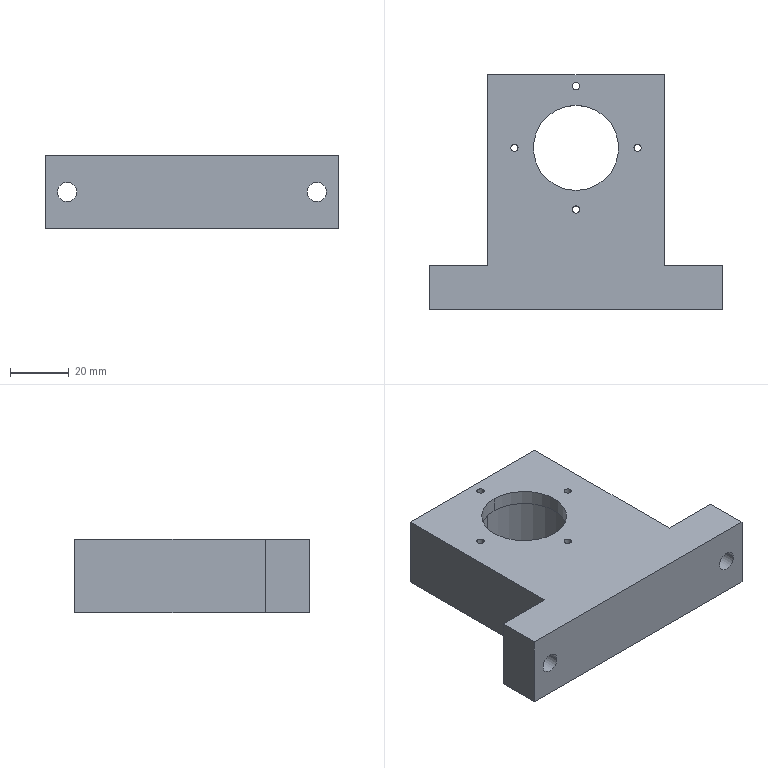Part | SolidWorks | features BaseBody 1 | 1 solid | 37 faces | box 100 x 80 x 25 mm | volume 110111 mm3 | cylinder 20 | plane 13 | cone 4 | commonest cylinder face diameters 2.5 x8 6.6 x4 11 x4 29 x2 35 x2
STEP:
#1=CARTESIAN_POINT('',(-22.25,7.5,25.));
#2=VERTEX_POINT('',#1);
#3=CARTESIAN_POINT('',(-19.75,7.5,25.));
#4=VERTEX_POINT('',#3);
#5=CARTESIAN_POINT('',(-21.,7.5,25.));
#6=DIRECTION('',(0.,0.,1.));
#7=DIRECTION('',(-1.,0.,0.));
#8=AXIS2_PLACEMENT_3D('',#5,#6,#7);
#9=CIRCLE('',#8,1.25);
#10=EDGE_CURVE('',#2,#4,#9,.T.);
#11=ORIENTED_EDGE('',*,*,#10,.T.);
#12=CARTESIAN_POINT('',(-19.75,7.5,0.));
#13=VERTEX_POINT('',#12);
#14=CARTESIAN_POINT('',(-19.75,7.5,25.));
#15=DIRECTION('',(0.,0.,-1.));
#16=VECTOR('',#15,1000.);
#17=LINE('',#14,#16);
#18=EDGE_CURVE('',#4,#13,#17,.T.);
#19=ORIENTED_EDGE('',*,*,#18,.T.);
#20=CARTESIAN_POINT('',(-22.25,7.5,0.));
#21=VERTEX_POINT('',#20);
#22=CARTESIAN_POINT('',(-21.,7.5,0.));
#23=DIRECTION('',(0.,0.,-1.));
#24=DIRECTION('',(-1.,0.,0.));
#25=AXIS2_PLACEMENT_3D('',#22,#23,#24);
#26=CIRCLE('',#25,1.25);
#27=EDGE_CURVE('',#13,#21,#26,.T.);
#28=ORIENTED_EDGE('',*,*,#27,.T.);
#29=CARTESIAN_POINT('',(-22.25,7.5,25.));
#30=DIRECTION('',(0.,0.,-1.));
#31=VECTOR('',#30,1000.);
#32=LINE('',#29,#31);
#33=EDGE_CURVE('',#2,#21,#32,.T.);
#34=ORIENTED_EDGE('',*,*,#33,.F.);
#35=EDGE_LOOP('',(#11,#19,#28,#34));
#36=FACE_OUTER_BOUND('',#35,.T.);
#37=CARTESIAN_POINT('',(-21.,7.5,25.));
#38=DIRECTION('',(0.,0.,-1.));
#39=DIRECTION('',(-1.,0.,0.));
#40=AXIS2_PLACEMENT_3D('',#37,#38,#39);
#41=CYLINDRICAL_SURFACE('',#40,1.25);
#42=ADVANCED_FACE('',(#36),#41,.F.);
#43=CARTESIAN_POINT('',(0.,25.,20.));
#44=VERTEX_POINT('',#43);
#45=CARTESIAN_POINT('',(0.,-10.,20.));
#46=VERTEX_POINT('',#45);
#47=CARTESIAN_POINT('',(0.,7.5,20.));
#48=DIRECTION('',(0.,0.,1.));
#49=DIRECTION('',(0.,1.,0.));
#50=AXIS2_PLACEMENT_3D('',#47,#48,#49);
#51=CIRCLE('',#50,17.5);
#52=EDGE_CURVE('',#44,#46,#51,.T.);
#53=ORIENTED_EDGE('',*,*,#52,.T.);
#54=CARTESIAN_POINT('',(0.,-10.,0.));
#55=VERTEX_POINT('',#54);
#56=CARTESIAN_POINT('',(0.,-10.,20.));
#57=DIRECTION('',(0.,0.,-1.));
#58=VECTOR('',#57,1000.);
#59=LINE('',#56,#58);
#60=EDGE_CURVE('',#46,#55,#59,.T.);
#61=ORIENTED_EDGE('',*,*,#60,.T.);
#62=CARTESIAN_POINT('',(0.,25.,0.));
#63=VERTEX_POINT('',#62);
#64=CARTESIAN_POINT('',(0.,7.5,0.));
#65=DIRECTION('',(0.,0.,-1.));
#66=DIRECTION('',(0.,1.,0.));
#67=AXIS2_PLACEMENT_3D('',#64,#65,#66);
#68=CIRCLE('',#67,17.5);
#69=EDGE_CURVE('',#55,#63,#68,.T.);
#70=ORIENTED_EDGE('',*,*,#69,.T.);
#71=CARTESIAN_POINT('',(0.,25.,20.));
#72=DIRECTION('',(0.,0.,-1.));
#73=VECTOR('',#72,1000.);
#74=LINE('',#71,#73);
#75=EDGE_CURVE('',#44,#63,#74,.T.);
#76=ORIENTED_EDGE('',*,*,#75,.F.);
#77=EDGE_LOOP('',(#53,#61,#70,#76));
#78=FACE_OUTER_BOUND('',#77,.T.);
#79=CARTESIAN_POINT('',(0.,7.5,20.));
#80=DIRECTION('',(0.,0.,-1.));
#81=DIRECTION('',(0.,1.,0.));
#82=AXIS2_PLACEMENT_3D('',#79,#80,#81);
#83=CYLINDRICAL_SURFACE('',#82,17.5);
#84=ADVANCED_FACE('',(#78),#83,.F.);
#85=CARTESIAN_POINT('',(1.25,28.5,25.));
#86=VERTEX_POINT('',#85);
#87=CARTESIAN_POINT('',(-1.25,28.5,25.));
#88=VERTEX_POINT('',#87);
#89=CARTESIAN_POINT('',(0.,28.5,25.));
#90=DIRECTION('',(0.,0.,-1.));
#91=DIRECTION('',(-1.,0.,0.));
#92=AXIS2_PLACEMENT_3D('',#89,#90,#91);
#93=CIRCLE('',#92,1.25);
#94=EDGE_CURVE('',#86,#88,#93,.T.);
#95=ORIENTED_EDGE('',*,*,#94,.F.);
#96=CARTESIAN_POINT('',(1.25,28.5,0.));
#97=VERTEX_POINT('',#96);
#98=CARTESIAN_POINT('',(1.25,28.5,25.));
#99=DIRECTION('',(0.,0.,-1.));
#100=VECTOR('',#99,1000.);
#101=LINE('',#98,#100);
#102=EDGE_CURVE('',#86,#97,#101,.T.);
#103=ORIENTED_EDGE('',*,*,#102,.T.);
#104=CARTESIAN_POINT('',(-1.25,28.5,0.));
#105=VERTEX_POINT('',#104);
#106=CARTESIAN_POINT('',(0.,28.5,0.));
#107=DIRECTION('',(0.,0.,-1.));
#108=DIRECTION('',(-1.,0.,0.));
#109=AXIS2_PLACEMENT_3D('',#106,#107,#108);
#110=CIRCLE('',#109,1.25);
#111=EDGE_CURVE('',#97,#105,#110,.T.);
#112=ORIENTED_EDGE('',*,*,#111,.T.);
#113=CARTESIAN_POINT('',(-1.25,28.5,25.));
#114=DIRECTION('',(0.,0.,-1.));
#115=VECTOR('',#114,1000.);
#116=LINE('',#113,#115);
#117=EDGE_CURVE('',#88,#105,#116,.T.);
#118=ORIENTED_EDGE('',*,*,#117,.F.);
#119=EDGE_LOOP('',(#95,#103,#112,#118));
#120=FACE_OUTER_BOUND('',#119,.T.);
#121=CARTESIAN_POINT('',(0.,28.5,25.));
#122=DIRECTION('',(0.,0.,-1.));
#123=DIRECTION('',(-1.,0.,0.));
#124=AXIS2_PLACEMENT_3D('',#121,#122,#123);
#125=CYLINDRICAL_SURFACE('',#124,1.25);
#126=ADVANCED_FACE('',(#120),#125,.F.);
#127=CARTESIAN_POINT('',(22.25,7.5,25.));
#128=VERTEX_POINT('',#127);
#129=CARTESIAN_POINT('',(19.75,7.5,25.));
#130=VERTEX_POINT('',#129);
#131=CARTESIAN_POINT('',(21.,7.5,25.));
#132=DIRECTION('',(0.,0.,-1.));
#133=DIRECTION('',(-1.,0.,0.));
#134=AXIS2_PLACEMENT_3D('',#131,#132,#133);
#135=CIRCLE('',#134,1.25);
#136=EDGE_CURVE('',#128,#130,#135,.T.);
#137=ORIENTED_EDGE('',*,*,#136,.F.);
#138=CARTESIAN_POINT('',(22.25,7.5,0.));
#139=VERTEX_POINT('',#138);
#140=CARTESIAN_POINT('',(22.25,7.5,25.));
#141=DIRECTION('',(0.,0.,-1.));
#142=VECTOR('',#141,1000.);
#143=LINE('',#140,#142);
#144=EDGE_CURVE('',#128,#139,#143,.T.);
#145=ORIENTED_EDGE('',*,*,#144,.T.);
#146=CARTESIAN_POINT('',(19.75,7.5,0.));
#147=VERTEX_POINT('',#146);
#148=CARTESIAN_POINT('',(21.,7.5,0.));
#149=DIRECTION('',(0.,0.,-1.));
#150=DIRECTION('',(-1.,0.,0.));
#151=AXIS2_PLACEMENT_3D('',#148,#149,#150);
#152=CIRCLE('',#151,1.25);
#153=EDGE_CURVE('',#139,#147,#152,.T.);
#154=ORIENTED_EDGE('',*,*,#153,.T.);
#155=CARTESIAN_POINT('',(19.75,7.5,25.));
#156=DIRECTION('',(0.,0.,-1.));
#157=VECTOR('',#156,1000.);
#158=LINE('',#155,#157);
#159=EDGE_CURVE('',#130,#147,#158,.T.);
#160=ORIENTED_EDGE('',*,*,#159,.F.);
#161=EDGE_LOOP('',(#137,#145,#154,#160));
#162=FACE_OUTER_BOUND('',#161,.T.);
#163=CARTESIAN_POINT('',(21.,7.5,25.));
#164=DIRECTION('',(0.,0.,-1.));
#165=DIRECTION('',(-1.,0.,0.));
#166=AXIS2_PLACEMENT_3D('',#163,#164,#165);
#167=CYLINDRICAL_SURFACE('',#166,1.25);
#168=ADVANCED_FACE('',(#162),#167,.F.);
#169=CARTESIAN_POINT('',(1.25,-13.5,25.));
#170=VERTEX_POINT('',#169);
#171=CARTESIAN_POINT('',(-1.25,-13.5,25.));
#172=VERTEX_POINT('',#171);
#173=CARTESIAN_POINT('',(0.,-13.5,25.));
#174=DIRECTION('',(0.,0.,-1.));
#175=DIRECTION('',(-1.,0.,0.));
#176=AXIS2_PLACEMENT_3D('',#173,#174,#175);
#177=CIRCLE('',#176,1.25);
#178=EDGE_CURVE('',#170,#172,#177,.T.);
#179=ORIENTED_EDGE('',*,*,#178,.F.);
#180=CARTESIAN_POINT('',(1.25,-13.5,0.));
#181=VERTEX_POINT('',#180);
#182=CARTESIAN_POINT('',(1.25,-13.5,25.));
#183=DIRECTION('',(0.,0.,-1.));
#184=VECTOR('',#183,1000.);
#185=LINE('',#182,#184);
#186=EDGE_CURVE('',#170,#181,#185,.T.);
#187=ORIENTED_EDGE('',*,*,#186,.T.);
#188=CARTESIAN_POINT('',(-1.25,-13.5,0.));
#189=VERTEX_POINT('',#188);
#190=CARTESIAN_POINT('',(0.,-13.5,0.));
#191=DIRECTION('',(0.,0.,-1.));
#192=DIRECTION('',(-1.,0.,0.));
#193=AXIS2_PLACEMENT_3D('',#190,#191,#192);
#194=CIRCLE('',#193,1.25);
#195=EDGE_CURVE('',#181,#189,#194,.T.);
#196=ORIENTED_EDGE('',*,*,#195,.T.);
#197=CARTESIAN_POINT('',(-1.25,-13.5,25.));
#198=DIRECTION('',(0.,0.,-1.));
#199=VECTOR('',#198,1000.);
#200=LINE('',#197,#199);
#201=EDGE_CURVE('',#172,#189,#200,.T.);
#202=ORIENTED_EDGE('',*,*,#201,.F.);
#203=EDGE_LOOP('',(#179,#187,#196,#202));
#204=FACE_OUTER_BOUND('',#203,.T.);
#205=CARTESIAN_POINT('',(0.,-13.5,25.));
#206=DIRECTION('',(0.,0.,-1.));
#207=DIRECTION('',(-1.,0.,0.));
#208=AXIS2_PLACEMENT_3D('',#205,#206,#207);
#209=CYLINDRICAL_SURFACE('',#208,1.25);
#210=ADVANCED_FACE('',(#204),#209,.F.);
#211=CARTESIAN_POINT('',(0.,-7.,20.));
#212=VERTEX_POINT('',#211);
#213=CARTESIAN_POINT('',(0.,22.,20.));
#214=VERTEX_POINT('',#213);
#215=CARTESIAN_POINT('',(0.,7.5,20.));
#216=DIRECTION('',(0.,0.,-1.));
#217=DIRECTION('',(0.,-1.,0.));
#218=AXIS2_PLACEMENT_3D('',#215,#216,#217);
#219=CIRCLE('',#218,14.5);
#220=EDGE_CURVE('',#212,#214,#219,.T.);
#221=ORIENTED_EDGE('',*,*,#220,.T.);
#222=CARTESIAN_POINT('',(0.,22.,25.));
#223=VERTEX_POINT('',#222);
#224=CARTESIAN_POINT('',(0.,22.,20.));
#225=DIRECTION('',(0.,0.,1.));
#226=VECTOR('',#225,1000.);
#227=LINE('',#224,#226);
#228=EDGE_CURVE('',#214,#223,#227,.T.);
#229=ORIENTED_EDGE('',*,*,#228,.T.);
#230=CARTESIAN_POINT('',(0.,-7.,25.));
#231=VERTEX_POINT('',#230);
#232=CARTESIAN_POINT('',(0.,7.5,25.));
#233=DIRECTION('',(0.,0.,-1.));
#234=DIRECTION('',(0.,-1.,0.));
#235=AXIS2_PLACEMENT_3D('',#232,#233,#234);
#236=CIRCLE('',#235,14.5);
#237=EDGE_CURVE('',#231,#223,#236,.T.);
#238=ORIENTED_EDGE('',*,*,#237,.F.);
#239=CARTESIAN_POINT('',(0.,-7.,20.));
#240=DIRECTION('',(0.,0.,1.));
#241=VECTOR('',#240,1000.);
#242=LINE('',#239,#241);
#243=EDGE_CURVE('',#212,#231,#242,.T.);
#244=ORIENTED_EDGE('',*,*,#243,.F.);
#245=EDGE_LOOP('',(#221,#229,#238,#244));
#246=FACE_OUTER_BOUND('',#245,.T.);
#247=CARTESIAN_POINT('',(0.,7.5,20.));
#248=DIRECTION('',(0.,0.,1.));
#249=DIRECTION('',(0.,-1.,0.));
#250=AXIS2_PLACEMENT_3D('',#247,#248,#249);
#251=CYLINDRICAL_SURFACE('',#250,14.5);
#252=ADVANCED_FACE('',(#246),#251,.F.);
#253=CARTESIAN_POINT('',(37.,-32.525,12.5));
#254=VERTEX_POINT('',#253);
#255=CARTESIAN_POINT('',(42.5,-32.525,7.));
#256=VERTEX_POINT('',#255);
#257=CARTESIAN_POINT('',(42.5,-32.525,12.5));
#258=DIRECTION('',(0.,-1.,0.));
#259=DIRECTION('',(0.,0.,1.));
#260=AXIS2_PLACEMENT_3D('',#257,#258,#259);
#261=CIRCLE('',#260,5.5);
#262=EDGE_CURVE('',#254,#256,#261,.T.);
#263=ORIENTED_EDGE('',*,*,#262,.T.);
#264=CARTESIAN_POINT('',(42.5,-32.5,6.975));
#265=VERTEX_POINT('',#264);
#266=CARTESIAN_POINT('',(42.5,-32.525,7.));
#267=DIRECTION('',(0.,0.7071,-0.7071));
#268=VECTOR('',#267,1000.);
#269=LINE('',#266,#268);
#270=EDGE_CURVE('',#256,#265,#269,.T.);
#271=ORIENTED_EDGE('',*,*,#270,.T.);
#272=CARTESIAN_POINT('',(42.5,-32.5,18.025));
#273=VERTEX_POINT('',#272);
#274=CARTESIAN_POINT('',(42.5,-32.5,12.5));
#275=DIRECTION('',(0.,1.,0.));
#276=DIRECTION('',(0.,0.,1.));
#277=AXIS2_PLACEMENT_3D('',#274,#275,#276);
#278=CIRCLE('',#277,5.525);
#279=EDGE_CURVE('',#265,#273,#278,.T.);
#280=ORIENTED_EDGE('',*,*,#279,.T.);
#281=CARTESIAN_POINT('',(42.5,-32.525,18.));
#282=VERTEX_POINT('',#281);
#283=CARTESIAN_POINT('',(42.5,-32.525,18.));
#284=DIRECTION('',(0.,0.7071,0.7071));
#285=VECTOR('',#284,1000.);
#286=LINE('',#283,#285);
#287=EDGE_CURVE('',#282,#273,#286,.T.);
#288=ORIENTED_EDGE('',*,*,#287,.F.);
#289=CARTESIAN_POINT('',(42.5,-32.525,12.5));
#290=DIRECTION('',(0.,-1.,0.));
#291=DIRECTION('',(0.,0.,1.));
#292=AXIS2_PLACEMENT_3D('',#289,#290,#291);
#293=CIRCLE('',#292,5.5);
#294=EDGE_CURVE('',#282,#254,#293,.T.);
#295=ORIENTED_EDGE('',*,*,#294,.T.);
#296=EDGE_LOOP('',(#263,#271,#280,#288,#295));
#297=FACE_OUTER_BOUND('',#296,.T.);
#298=CARTESIAN_POINT('',(42.5,-32.525,12.5));
#299=DIRECTION('',(0.,1.,0.));
#300=DIRECTION('',(0.,0.,1.));
#301=AXIS2_PLACEMENT_3D('',#298,#299,#300);
#302=CONICAL_SURFACE('',#301,5.5,0.7854);
#303=ADVANCED_FACE('',(#297),#302,.F.);
#304=CARTESIAN_POINT('',(45.8,-47.5,12.5));
#305=VERTEX_POINT('',#304);
#306=CARTESIAN_POINT('',(39.2,-47.5,12.5));
#307=VERTEX_POINT('',#306);
#308=CARTESIAN_POINT('',(42.5,-47.5,12.5));
#309=DIRECTION('',(0.,1.,0.));
#310=DIRECTION('',(-1.,0.,0.));
#311=AXIS2_PLACEMENT_3D('',#308,#309,#310);
#312=CIRCLE('',#311,3.3);
#313=EDGE_CURVE('',#305,#307,#312,.T.);
#314=ORIENTED_EDGE('',*,*,#313,.F.);
#315=CARTESIAN_POINT('',(45.8,-39.3,12.5));
#316=VERTEX_POINT('',#315);
#317=CARTESIAN_POINT('',(45.8,-47.5,12.5));
#318=DIRECTION('',(0.,1.,0.));
#319=VECTOR('',#318,1000.);
#320=LINE('',#317,#319);
#321=EDGE_CURVE('',#305,#316,#320,.T.);
#322=ORIENTED_EDGE('',*,*,#321,.T.);
#323=CARTESIAN_POINT('',(39.2,-39.3,12.5));
#324=VERTEX_POINT('',#323);
#325=CARTESIAN_POINT('',(42.5,-39.3,12.5));
#326=DIRECTION('',(0.,1.,0.));
#327=DIRECTION('',(-1.,0.,0.));
#328=AXIS2_PLACEMENT_3D('',#325,#326,#327);
#329=CIRCLE('',#328,3.3);
#330=EDGE_CURVE('',#316,#324,#329,.T.);
#331=ORIENTED_EDGE('',*,*,#330,.T.);
#332=CARTESIAN_POINT('',(39.2,-47.5,12.5));
#333=DIRECTION('',(0.,1.,0.));
#334=VECTOR('',#333,1000.);
#335=LINE('',#332,#334);
#336=EDGE_CURVE('',#307,#324,#335,.T.);
#337=ORIENTED_EDGE('',*,*,#336,.F.);
#338=EDGE_LOOP('',(#314,#322,#331,#337));
#339=FACE_OUTER_BOUND('',#338,.T.);
#340=CARTESIAN_POINT('',(42.5,-47.5,12.5));
#341=DIRECTION('',(0.,1.,0.));
#342=DIRECTION('',(-1.,0.,0.));
#343=AXIS2_PLACEMENT_3D('',#340,#341,#342);
#344=CYLINDRICAL_SURFACE('',#343,3.3);
#345=ADVANCED_FACE('',(#339),#344,.F.);
#346=CARTESIAN_POINT('',(-39.2,-47.5,12.5));
#347=VERTEX_POINT('',#346);
#348=CARTESIAN_POINT('',(-45.8,-47.5,12.5));
#349=VERTEX_POINT('',#348);
#350=CARTESIAN_POINT('',(-42.5,-47.5,12.5));
#351=DIRECTION('',(0.,1.,0.));
#352=DIRECTION('',(-1.,0.,0.));
#353=AXIS2_PLACEMENT_3D('',#350,#351,#352);
#354=CIRCLE('',#353,3.3);
#355=EDGE_CURVE('',#347,#349,#354,.T.);
#356=ORIENTED_EDGE('',*,*,#355,.F.);
#357=CARTESIAN_POINT('',(-39.2,-39.3,12.5));
#358=VERTEX_POINT('',#357);
#359=CARTESIAN_POINT('',(-39.2,-47.5,12.5));
#360=DIRECTION('',(0.,1.,0.));
#361=VECTOR('',#360,1000.);
#362=LINE('',#359,#361);
#363=EDGE_CURVE('',#347,#358,#362,.T.);
#364=ORIENTED_EDGE('',*,*,#363,.T.);
#365=CARTESIAN_POINT('',(-45.8,-39.3,12.5));
#366=VERTEX_POINT('',#365);
#367=CARTESIAN_POINT('',(-42.5,-39.3,12.5));
#368=DIRECTION('',(0.,1.,0.));
#369=DIRECTION('',(-1.,0.,0.));
#370=AXIS2_PLACEMENT_3D('',#367,#368,#369);
#371=CIRCLE('',#370,3.3);
#372=EDGE_CURVE('',#358,#366,#371,.T.);
#373=ORIENTED_EDGE('',*,*,#372,.T.);
#374=CARTESIAN_POINT('',(-45.8,-47.5,12.5));
#375=DIRECTION('',(0.,1.,0.));
#376=VECTOR('',#375,1000.);
#377=LINE('',#374,#376);
#378=EDGE_CURVE('',#349,#366,#377,.T.);
#379=ORIENTED_EDGE('',*,*,#378,.F.);
#380=EDGE_LOOP('',(#356,#364,#373,#379));
#381=FACE_OUTER_BOUND('',#380,.T.);
#382=CARTESIAN_POINT('',(-42.5,-47.5,12.5));
#383=DIRECTION('',(0.,1.,0.));
#384=DIRECTION('',(-1.,0.,0.));
#385=AXIS2_PLACEMENT_3D('',#382,#383,#384);
#386=CYLINDRICAL_SURFACE('',#385,3.3);
#387=ADVANCED_FACE('',(#381),#386,.F.);
#388=CARTESIAN_POINT('',(-48.,-32.525,12.5));
#389=VERTEX_POINT('',#388);
#390=CARTESIAN_POINT('',(-42.5,-32.525,7.));
#391=VERTEX_POINT('',#390);
#392=CARTESIAN_POINT('',(-42.5,-32.525,12.5));
#393=DIRECTION('',(0.,-1.,0.));
#394=DIRECTION('',(0.,0.,1.));
#395=AXIS2_PLACEMENT_3D('',#392,#393,#394);
#396=CIRCLE('',#395,5.5);
#397=EDGE_CURVE('',#389,#391,#396,.T.);
#398=ORIENTED_EDGE('',*,*,#397,.T.);
#399=CARTESIAN_POINT('',(-42.5,-32.5,6.975));
#400=VERTEX_POINT('',#399);
#401=CARTESIAN_POINT('',(-42.5,-32.525,7.));
#402=DIRECTION('',(0.,0.7071,-0.7071));
#403=VECTOR('',#402,1000.);
#404=LINE('',#401,#403);
#405=EDGE_CURVE('',#391,#400,#404,.T.);
#406=ORIENTED_EDGE('',*,*,#405,.T.);
#407=CARTESIAN_POINT('',(-42.5,-32.5,18.025));
#408=VERTEX_POINT('',#407);
#409=CARTESIAN_POINT('',(-42.5,-32.5,12.5));
#410=DIRECTION('',(0.,1.,0.));
#411=DIRECTION('',(0.,0.,1.));
#412=AXIS2_PLACEMENT_3D('',#409,#410,#411);
#413=CIRCLE('',#412,5.525);
#414=EDGE_CURVE('',#400,#408,#413,.T.);
#415=ORIENTED_EDGE('',*,*,#414,.T.);
#416=CARTESIAN_POINT('',(-42.5,-32.525,18.));
#417=VERTEX_POINT('',#416);
#418=CARTESIAN_POINT('',(-42.5,-32.525,18.));
#419=DIRECTION('',(0.,0.7071,0.7071));
#420=VECTOR('',#419,1000.);
#421=LINE('',#418,#420);
#422=EDGE_CURVE('',#417,#408,#421,.T.);
#423=ORIENTED_EDGE('',*,*,#422,.F.);
#424=CARTESIAN_POINT('',(-42.5,-32.525,12.5));
#425=DIRECTION('',(0.,-1.,0.));
#426=DIRECTION('',(0.,0.,1.));
#427=AXIS2_PLACEMENT_3D('',#424,#425,#426);
#428=CIRCLE('',#427,5.5);
#429=EDGE_CURVE('',#417,#389,#428,.T.);
#430=ORIENTED_EDGE('',*,*,#429,.T.);
#431=EDGE_LOOP('',(#398,#406,#415,#423,#430));
#432=FACE_OUTER_BOUND('',#431,.T.);
#433=CARTESIAN_POINT('',(-42.5,-32.525,12.5));
#434=DIRECTION('',(0.,1.,0.));
#435=DIRECTION('',(0.,0.,1.));
#436=AXIS2_PLACEMENT_3D('',#433,#434,#435);
#437=CONICAL_SURFACE('',#436,5.5,0.7854);
#438=ADVANCED_FACE('',(#432),#437,.F.);
#439=CARTESIAN_POINT('',(37.,-39.3,12.5));
#440=VERTEX_POINT('',#439);
#441=CARTESIAN_POINT('',(48.,-39.3,12.5));
#442=VERTEX_POINT('',#441);
#443=CARTESIAN_POINT('',(42.5,-39.3,12.5));
#444=DIRECTION('',(0.,-1.,0.));
#445=DIRECTION('',(-1.,0.,0.));
#446=AXIS2_PLACEMENT_3D('',#443,#444,#445);
#447=CIRCLE('',#446,5.5);
#448=EDGE_CURVE('',#440,#442,#447,.T.);
#449=ORIENTED_EDGE('',*,*,#448,.T.);
#450=CARTESIAN_POINT('',(48.,-32.525,12.5));
#451=VERTEX_POINT('',#450);
#452=CARTESIAN_POINT('',(48.,-39.3,12.5));
#453=DIRECTION('',(0.,1.,0.));
#454=VECTOR('',#453,1000.);
#455=LINE('',#452,#454);
#456=EDGE_CURVE('',#442,#451,#455,.T.);
#457=ORIENTED_EDGE('',*,*,#456,.T.);
#458=CARTESIAN_POINT('',(42.5,-32.525,12.5));
#459=DIRECTION('',(0.,-1.,0.));
#460=DIRECTION('',(0.,0.,1.));
#461=AXIS2_PLACEMENT_3D('',#458,#459,#460);
#462=CIRCLE('',#461,5.5);
#463=EDGE_CURVE('',#256,#451,#462,.T.);
#464=ORIENTED_EDGE('',*,*,#463,.F.);
#465=ORIENTED_EDGE('',*,*,#262,.F.);
#466=CARTESIAN_POINT('',(37.,-39.3,12.5));
#467=DIRECTION('',(0.,1.,0.));
#468=VECTOR('',#467,1000.);
#469=LINE('',#466,#468);
#470=EDGE_CURVE('',#440,#254,#469,.T.);
#471=ORIENTED_EDGE('',*,*,#470,.F.);
#472=EDGE_LOOP('',(#449,#457,#464,#465,#471));
#473=FACE_OUTER_BOUND('',#472,.T.);
#474=CARTESIAN_POINT('',(42.5,-39.3,12.5));
#475=DIRECTION('',(0.,1.,0.));
#476=DIRECTION('',(-1.,0.,0.));
#477=AXIS2_PLACEMENT_3D('',#474,#475,#476);
#478=CYLINDRICAL_SURFACE('',#477,5.5);
#479=ADVANCED_FACE('',(#473),#478,.F.);
#480=CARTESIAN_POINT('',(-48.,-39.3,12.5));
#481=VERTEX_POINT('',#480);
#482=CARTESIAN_POINT('',(-37.,-39.3,12.5));
#483=VERTEX_POINT('',#482);
#484=CARTESIAN_POINT('',(-42.5,-39.3,12.5));
#485=DIRECTION('',(0.,-1.,0.));
#486=DIRECTION('',(-1.,0.,0.));
#487=AXIS2_PLACEMENT_3D('',#484,#485,#486);
#488=CIRCLE('',#487,5.5);
#489=EDGE_CURVE('',#481,#483,#488,.T.);
#490=ORIENTED_EDGE('',*,*,#489,.T.);
#491=CARTESIAN_POINT('',(-37.,-32.525,12.5));
#492=VERTEX_POINT('',#491);
#493=CARTESIAN_POINT('',(-37.,-39.3,12.5));
#494=DIRECTION('',(0.,1.,0.));
#495=VECTOR('',#494,1000.);
#496=LINE('',#493,#495);
#497=EDGE_CURVE('',#483,#492,#496,.T.);
#498=ORIENTED_EDGE('',*,*,#497,.T.);
#499=CARTESIAN_POINT('',(-42.5,-32.525,12.5));
#500=DIRECTION('',(0.,-1.,0.));
#501=DIRECTION('',(0.,0.,1.));
#502=AXIS2_PLACEMENT_3D('',#499,#500,#501);
#503=CIRCLE('',#502,5.5);
#504=EDGE_CURVE('',#391,#492,#503,.T.);
#505=ORIENTED_EDGE('',*,*,#504,.F.);
#506=ORIENTED_EDGE('',*,*,#397,.F.);
#507=CARTESIAN_POINT('',(-48.,-39.3,12.5));
#508=DIRECTION('',(0.,1.,0.));
#509=VECTOR('',#508,1000.);
#510=LINE('',#507,#509);
#511=EDGE_CURVE('',#481,#389,#510,.T.);
#512=ORIENTED_EDGE('',*,*,#511,.F.);
#513=EDGE_LOOP('',(#490,#498,#505,#506,#512));
#514=FACE_OUTER_BOUND('',#513,.T.);
#515=CARTESIAN_POINT('',(-42.5,-39.3,12.5));
#516=DIRECTION('',(0.,1.,0.));
#517=DIRECTION('',(-1.,0.,0.));
#518=AXIS2_PLACEMENT_3D('',#515,#516,#517);
#519=CYLINDRICAL_SURFACE('',#518,5.5);
#520=ADVANCED_FACE('',(#514),#519,.F.);
#521=ORIENTED_EDGE('',*,*,#18,.F.);
#522=CARTESIAN_POINT('',(-21.,7.5,25.));
#523=DIRECTION('',(0.,0.,1.));
#524=DIRECTION('',(-1.,0.,0.));
#525=AXIS2_PLACEMENT_3D('',#522,#523,#524);
#526=CIRCLE('',#525,1.25);
#527=EDGE_CURVE('',#4,#2,#526,.T.);
#528=ORIENTED_EDGE('',*,*,#527,.T.);
#529=ORIENTED_EDGE('',*,*,#33,.T.);
#530=CARTESIAN_POINT('',(-21.,7.5,0.));
#531=DIRECTION('',(0.,0.,-1.));
#532=DIRECTION('',(-1.,0.,0.));
#533=AXIS2_PLACEMENT_3D('',#530,#531,#532);
#534=CIRCLE('',#533,1.25);
#535=EDGE_CURVE('',#21,#13,#534,.T.);
#536=ORIENTED_EDGE('',*,*,#535,.T.);
#537=EDGE_LOOP('',(#521,#528,#529,#536));
#538=FACE_OUTER_BOUND('',#537,.T.);
#539=CARTESIAN_POINT('',(-21.,7.5,25.));
#540=DIRECTION('',(0.,0.,-1.));
#541=DIRECTION('',(-1.,0.,0.));
#542=AXIS2_PLACEMENT_3D('',#539,#540,#541);
#543=CYLINDRICAL_SURFACE('',#542,1.25);
#544=ADVANCED_FACE('',(#538),#543,.F.);
#545=CARTESIAN_POINT('',(0.,7.5,0.));
#546=DIRECTION('',(0.,0.,-1.));
#547=DIRECTION('',(0.,1.,0.));
#548=AXIS2_PLACEMENT_3D('',#545,#546,#547);
#549=CIRCLE('',#548,17.5);
#550=EDGE_CURVE('',#63,#55,#549,.T.);
#551=ORIENTED_EDGE('',*,*,#550,.F.);
#552=ORIENTED_EDGE('',*,*,#69,.F.);
#553=EDGE_LOOP('',(#551,#552));
#554=FACE_BOUND('',#553,.T.);
#555=CARTESIAN_POINT('',(0.,28.5,0.));
#556=DIRECTION('',(0.,0.,-1.));
#557=DIRECTION('',(-1.,0.,0.));
#558=AXIS2_PLACEMENT_3D('',#555,#556,#557);
#559=CIRCLE('',#558,1.25);
#560=EDGE_CURVE('',#105,#97,#559,.T.);
#561=ORIENTED_EDGE('',*,*,#560,.F.);
#562=ORIENTED_EDGE('',*,*,#111,.F.);
#563=EDGE_LOOP('',(#561,#562));
#564=FACE_BOUND('',#563,.T.);
#565=CARTESIAN_POINT('',(21.,7.5,0.));
#566=DIRECTION('',(0.,0.,-1.));
#567=DIRECTION('',(-1.,0.,0.));
#568=AXIS2_PLACEMENT_3D('',#565,#566,#567);
#569=CIRCLE('',#568,1.25);
#570=EDGE_CURVE('',#147,#139,#569,.T.);
#571=ORIENTED_EDGE('',*,*,#570,.F.);
#572=ORIENTED_EDGE('',*,*,#153,.F.);
#573=EDGE_LOOP('',(#571,#572));
#574=FACE_BOUND('',#573,.T.);
#575=CARTESIAN_POINT('',(0.,-13.5,0.));
#576=DIRECTION('',(0.,0.,-1.));
#577=DIRECTION('',(-1.,0.,0.));
#578=AXIS2_PLACEMENT_3D('',#575,#576,#577);
#579=CIRCLE('',#578,1.25);
#580=EDGE_CURVE('',#189,#181,#579,.T.);
#581=ORIENTED_EDGE('',*,*,#580,.F.);
#582=ORIENTED_EDGE('',*,*,#195,.F.);
#583=EDGE_LOOP('',(#581,#582));
#584=FACE_BOUND('',#583,.T.);
#585=ORIENTED_EDGE('',*,*,#535,.F.);
#586=ORIENTED_EDGE('',*,*,#27,.F.);
#587=EDGE_LOOP('',(#585,#586));
#588=FACE_BOUND('',#587,.T.);
#589=CARTESIAN_POINT('',(50.,-32.5,0.));
#590=VERTEX_POINT('',#589);
#591=CARTESIAN_POINT('',(30.,-32.5,0.));
#592=VERTEX_POINT('',#591);
#593=CARTESIAN_POINT('',(0.,-32.5,0.));
#594=DIRECTION('',(-1.,0.,0.));
#595=VECTOR('',#594,1000.);
#596=LINE('',#593,#595);
#597=EDGE_CURVE('',#590,#592,#596,.T.);
#598=ORIENTED_EDGE('',*,*,#597,.F.);
#599=CARTESIAN_POINT('',(50.,-47.5,0.));
#600=VERTEX_POINT('',#599);
#601=CARTESIAN_POINT('',(50.,-7.5,0.));
#602=DIRECTION('',(0.,1.,0.));
#603=VECTOR('',#602,1000.);
#604=LINE('',#601,#603);
#605=EDGE_CURVE('',#600,#590,#604,.T.);
#606=ORIENTED_EDGE('',*,*,#605,.F.);
#607=CARTESIAN_POINT('',(-50.,-47.5,0.));
#608=VERTEX_POINT('',#607);
#609=CARTESIAN_POINT('',(0.,-47.5,0.));
#610=DIRECTION('',(1.,0.,0.));
#611=VECTOR('',#610,1000.);
#612=LINE('',#609,#611);
#613=EDGE_CURVE('',#608,#600,#612,.T.);
#614=ORIENTED_EDGE('',*,*,#613,.F.);
#615=CARTESIAN_POINT('',(-50.,-32.5,0.));
#616=VERTEX_POINT('',#615);
#617=CARTESIAN_POINT('',(-50.,-7.5,0.));
#618=DIRECTION('',(0.,-1.,0.));
#619=VECTOR('',#618,1000.);
#620=LINE('',#617,#619);
#621=EDGE_CURVE('',#616,#608,#620,.T.);
#622=ORIENTED_EDGE('',*,*,#621,.F.);
#623=CARTESIAN_POINT('',(-30.,-32.5,0.));
#624=VERTEX_POINT('',#623);
#625=CARTESIAN_POINT('',(0.,-32.5,0.));
#626=DIRECTION('',(-1.,0.,0.));
#627=VECTOR('',#626,1000.);
#628=LINE('',#625,#627);
#629=EDGE_CURVE('',#624,#616,#628,.T.);
#630=ORIENTED_EDGE('',*,*,#629,.F.);
#631=CARTESIAN_POINT('',(-30.,32.5,0.));
#632=VERTEX_POINT('',#631);
#633=CARTESIAN_POINT('',(-30.,-7.5,0.));
#634=DIRECTION('',(0.,-1.,0.));
#635=VECTOR('',#634,1000.);
#636=LINE('',#633,#635);
#637=EDGE_CURVE('',#632,#624,#636,.T.);
#638=ORIENTED_EDGE('',*,*,#637,.F.);
#639=CARTESIAN_POINT('',(30.,32.5,0.));
#640=VERTEX_POINT('',#639);
#641=CARTESIAN_POINT('',(0.,32.5,0.));
#642=DIRECTION('',(-1.,0.,0.));
#643=VECTOR('',#642,1000.);
#644=LINE('',#641,#643);
#645=EDGE_CURVE('',#640,#632,#644,.T.);
#646=ORIENTED_EDGE('',*,*,#645,.F.);
#647=CARTESIAN_POINT('',(30.,-7.5,0.));
#648=DIRECTION('',(0.,1.,0.));
#649=VECTOR('',#648,1000.);
#650=LINE('',#647,#649);
#651=EDGE_CURVE('',#592,#640,#650,.T.);
#652=ORIENTED_EDGE('',*,*,#651,.F.);
#653=EDGE_LOOP('',(#598,#606,#614,#622,#630,#638,#646,#652));
#654=FACE_OUTER_BOUND('',#653,.T.);
#655=CARTESIAN_POINT('',(-50.,-47.5,0.));
#656=DIRECTION('',(0.,0.,1.));
#657=DIRECTION('',(1.,0.,0.));
#658=AXIS2_PLACEMENT_3D('',#655,#656,#657);
#659=PLANE('',#658);
#660=ADVANCED_FACE('',(#554,#564,#574,#584,#588,#654),#659,.F.);
#661=ORIENTED_EDGE('',*,*,#237,.T.);
#662=CARTESIAN_POINT('',(0.,7.5,25.));
#663=DIRECTION('',(0.,0.,-1.));
#664=DIRECTION('',(0.,-1.,0.));
#665=AXIS2_PLACEMENT_3D('',#662,#663,#664);
#666=CIRCLE('',#665,14.5);
#667=EDGE_CURVE('',#223,#231,#666,.T.);
#668=ORIENTED_EDGE('',*,*,#667,.T.);
#669=EDGE_LOOP('',(#661,#668));
#670=FACE_BOUND('',#669,.T.);
#671=CARTESIAN_POINT('',(0.,28.5,25.));
#672=DIRECTION('',(0.,0.,-1.));
#673=DIRECTION('',(-1.,0.,0.));
#674=AXIS2_PLACEMENT_3D('',#671,#672,#673);
#675=CIRCLE('',#674,1.25);
#676=EDGE_CURVE('',#88,#86,#675,.T.);
#677=ORIENTED_EDGE('',*,*,#676,.T.);
#678=ORIENTED_EDGE('',*,*,#94,.T.);
#679=EDGE_LOOP('',(#677,#678));
#680=FACE_BOUND('',#679,.T.);
#681=CARTESIAN_POINT('',(21.,7.5,25.));
#682=DIRECTION('',(0.,0.,-1.));
#683=DIRECTION('',(-1.,0.,0.));
#684=AXIS2_PLACEMENT_3D('',#681,#682,#683);
#685=CIRCLE('',#684,1.25);
#686=EDGE_CURVE('',#130,#128,#685,.T.);
#687=ORIENTED_EDGE('',*,*,#686,.T.);
#688=ORIENTED_EDGE('',*,*,#136,.T.);
#689=EDGE_LOOP('',(#687,#688));
#690=FACE_BOUND('',#689,.T.);
#691=CARTESIAN_POINT('',(0.,-13.5,25.));
#692=DIRECTION('',(0.,0.,-1.));
#693=DIRECTION('',(-1.,0.,0.));
#694=AXIS2_PLACEMENT_3D('',#691,#692,#693);
#695=CIRCLE('',#694,1.25);
#696=EDGE_CURVE('',#172,#170,#695,.T.);
#697=ORIENTED_EDGE('',*,*,#696,.T.);
#698=ORIENTED_EDGE('',*,*,#178,.T.);
#699=EDGE_LOOP('',(#697,#698));
#700=FACE_BOUND('',#699,.T.);
#701=ORIENTED_EDGE('',*,*,#10,.F.);
#702=ORIENTED_EDGE('',*,*,#527,.F.);
#703=EDGE_LOOP('',(#701,#702));
#704=FACE_BOUND('',#703,.T.);
#705=CARTESIAN_POINT('',(50.,-47.5,25.));
#706=VERTEX_POINT('',#705);
#707=CARTESIAN_POINT('',(50.,-32.5,25.));
#708=VERTEX_POINT('',#707);
#709=CARTESIAN_POINT('',(50.,-7.5,25.));
#710=DIRECTION('',(0.,1.,0.));
#711=VECTOR('',#710,1000.);
#712=LINE('',#709,#711);
#713=EDGE_CURVE('',#706,#708,#712,.T.);
#714=ORIENTED_EDGE('',*,*,#713,.T.);
#715=CARTESIAN_POINT('',(30.,-32.5,25.));
#716=VERTEX_POINT('',#715);
#717=CARTESIAN_POINT('',(0.,-32.5,25.));
#718=DIRECTION('',(-1.,0.,0.));
#719=VECTOR('',#718,1000.);
#720=LINE('',#717,#719);
#721=EDGE_CURVE('',#708,#716,#720,.T.);
#722=ORIENTED_EDGE('',*,*,#721,.T.);
#723=CARTESIAN_POINT('',(30.,32.5,25.));
#724=VERTEX_POINT('',#723);
#725=CARTESIAN_POINT('',(30.,-7.5,25.));
#726=DIRECTION('',(0.,1.,0.));
#727=VECTOR('',#726,1000.);
#728=LINE('',#725,#727);
#729=EDGE_CURVE('',#716,#724,#728,.T.);
#730=ORIENTED_EDGE('',*,*,#729,.T.);
#731=CARTESIAN_POINT('',(-30.,32.5,25.));
#732=VERTEX_POINT('',#731);
#733=CARTESIAN_POINT('',(0.,32.5,25.));
#734=DIRECTION('',(-1.,0.,0.));
#735=VECTOR('',#734,1000.);
#736=LINE('',#733,#735);
#737=EDGE_CURVE('',#724,#732,#736,.T.);
#738=ORIENTED_EDGE('',*,*,#737,.T.);
#739=CARTESIAN_POINT('',(-30.,-32.5,25.));
#740=VERTEX_POINT('',#739);
#741=CARTESIAN_POINT('',(-30.,-7.5,25.));
#742=DIRECTION('',(0.,-1.,0.));
#743=VECTOR('',#742,1000.);
#744=LINE('',#741,#743);
#745=EDGE_CURVE('',#732,#740,#744,.T.);
#746=ORIENTED_EDGE('',*,*,#745,.T.);
#747=CARTESIAN_POINT('',(-50.,-32.5,25.));
#748=VERTEX_POINT('',#747);
#749=CARTESIAN_POINT('',(0.,-32.5,25.));
#750=DIRECTION('',(-1.,0.,0.));
#751=VECTOR('',#750,1000.);
#752=LINE('',#749,#751);
#753=EDGE_CURVE('',#740,#748,#752,.T.);
#754=ORIENTED_EDGE('',*,*,#753,.T.);
#755=CARTESIAN_POINT('',(-50.,-47.5,25.));
#756=VERTEX_POINT('',#755);
#757=CARTESIAN_POINT('',(-50.,-7.5,25.));
#758=DIRECTION('',(0.,-1.,0.));
#759=VECTOR('',#758,1000.);
#760=LINE('',#757,#759);
#761=EDGE_CURVE('',#748,#756,#760,.T.);
#762=ORIENTED_EDGE('',*,*,#761,.T.);
#763=CARTESIAN_POINT('',(0.,-47.5,25.));
#764=DIRECTION('',(1.,0.,0.));
#765=VECTOR('',#764,1000.);
#766=LINE('',#763,#765);
#767=EDGE_CURVE('',#756,#706,#766,.T.);
#768=ORIENTED_EDGE('',*,*,#767,.T.);
#769=EDGE_LOOP('',(#714,#722,#730,#738,#746,#754,#762,#768));
#770=FACE_OUTER_BOUND('',#769,.T.);
#771=CARTESIAN_POINT('',(-50.,-47.5,25.));
#772=DIRECTION('',(0.,0.,1.));
#773=DIRECTION('',(1.,0.,0.));
#774=AXIS2_PLACEMENT_3D('',#771,#772,#773);
#775=PLANE('',#774);
#776=ADVANCED_FACE('',(#670,#680,#690,#700,#704,#770),#775,.T.);
#777=ORIENTED_EDGE('',*,*,#60,.F.);
#778=CARTESIAN_POINT('',(0.,7.5,20.));
#779=DIRECTION('',(0.,0.,1.));
#780=DIRECTION('',(0.,1.,0.));
#781=AXIS2_PLACEMENT_3D('',#778,#779,#780);
#782=CIRCLE('',#781,17.5);
#783=EDGE_CURVE('',#46,#44,#782,.T.);
#784=ORIENTED_EDGE('',*,*,#783,.T.);
#785=ORIENTED_EDGE('',*,*,#75,.T.);
#786=ORIENTED_EDGE('',*,*,#550,.T.);
#787=EDGE_LOOP('',(#777,#784,#785,#786));
#788=FACE_OUTER_BOUND('',#787,.T.);
#789=CARTESIAN_POINT('',(0.,7.5,20.));
#790=DIRECTION('',(0.,0.,-1.));
#791=DIRECTION('',(0.,1.,0.));
#792=AXIS2_PLACEMENT_3D('',#789,#790,#791);
#793=CYLINDRICAL_SURFACE('',#792,17.5);
#794=ADVANCED_FACE('',(#788),#793,.F.);
#795=ORIENTED_EDGE('',*,*,#102,.F.);
#796=ORIENTED_EDGE('',*,*,#676,.F.);
#797=ORIENTED_EDGE('',*,*,#117,.T.);
#798=ORIENTED_EDGE('',*,*,#560,.T.);
#799=EDGE_LOOP('',(#795,#796,#797,#798));
#800=FACE_OUTER_BOUND('',#799,.T.);
#801=CARTESIAN_POINT('',(0.,28.5,25.));
#802=DIRECTION('',(0.,0.,-1.));
#803=DIRECTION('',(-1.,0.,0.));
#804=AXIS2_PLACEMENT_3D('',#801,#802,#803);
#805=CYLINDRICAL_SURFACE('',#804,1.25);
#806=ADVANCED_FACE('',(#800),#805,.F.);
#807=ORIENTED_EDGE('',*,*,#144,.F.);
#808=ORIENTED_EDGE('',*,*,#686,.F.);
#809=ORIENTED_EDGE('',*,*,#159,.T.);
#810=ORIENTED_EDGE('',*,*,#570,.T.);
#811=EDGE_LOOP('',(#807,#808,#809,#810));
#812=FACE_OUTER_BOUND('',#811,.T.);
#813=CARTESIAN_POINT('',(21.,7.5,25.));
#814=DIRECTION('',(0.,0.,-1.));
#815=DIRECTION('',(-1.,0.,0.));
#816=AXIS2_PLACEMENT_3D('',#813,#814,#815);
#817=CYLINDRICAL_SURFACE('',#816,1.25);
#818=ADVANCED_FACE('',(#812),#817,.F.);
#819=ORIENTED_EDGE('',*,*,#186,.F.);
#820=ORIENTED_EDGE('',*,*,#696,.F.);
#821=ORIENTED_EDGE('',*,*,#201,.T.);
#822=ORIENTED_EDGE('',*,*,#580,.T.);
#823=EDGE_LOOP('',(#819,#820,#821,#822));
#824=FACE_OUTER_BOUND('',#823,.T.);
#825=CARTESIAN_POINT('',(0.,-13.5,25.));
#826=DIRECTION('',(0.,0.,-1.));
#827=DIRECTION('',(-1.,0.,0.));
#828=AXIS2_PLACEMENT_3D('',#825,#826,#827);
#829=CYLINDRICAL_SURFACE('',#828,1.25);
#830=ADVANCED_FACE('',(#824),#829,.F.);
#831=CARTESIAN_POINT('',(30.,32.5,12.5));
#832=DIRECTION('',(0.,0.,-1.));
#833=VECTOR('',#832,1000.);
#834=LINE('',#831,#833);
#835=EDGE_CURVE('',#724,#640,#834,.T.);
#836=ORIENTED_EDGE('',*,*,#835,.F.);
#837=ORIENTED_EDGE('',*,*,#729,.F.);
#838=CARTESIAN_POINT('',(30.,-32.5,12.5));
#839=DIRECTION('',(0.,0.,1.));
#840=VECTOR('',#839,1000.);
#841=LINE('',#838,#840);
#842=EDGE_CURVE('',#592,#716,#841,.T.);
#843=ORIENTED_EDGE('',*,*,#842,.F.);
#844=ORIENTED_EDGE('',*,*,#651,.T.);
#845=EDGE_LOOP('',(#836,#837,#843,#844));
#846=FACE_OUTER_BOUND('',#845,.T.);
#847=CARTESIAN_POINT('',(30.,32.5,0.));
#848=DIRECTION('',(-1.,0.,0.));
#849=DIRECTION('',(0.,-1.,0.));
#850=AXIS2_PLACEMENT_3D('',#847,#848,#849);
#851=PLANE('',#850);
#852=ADVANCED_FACE('',(#846),#851,.F.);
#853=CARTESIAN_POINT('',(42.5,-32.5,12.5));
#854=DIRECTION('',(0.,1.,0.));
#855=DIRECTION('',(0.,0.,1.));
#856=AXIS2_PLACEMENT_3D('',#853,#854,#855);
#857=CIRCLE('',#856,5.525);
#858=EDGE_CURVE('',#273,#265,#857,.T.);
#859=ORIENTED_EDGE('',*,*,#858,.F.);
#860=ORIENTED_EDGE('',*,*,#279,.F.);
#861=EDGE_LOOP('',(#859,#860));
#862=FACE_BOUND('',#861,.T.);
#863=ORIENTED_EDGE('',*,*,#721,.F.);
#864=CARTESIAN_POINT('',(50.,-32.5,12.5));
#865=DIRECTION('',(0.,0.,1.));
#866=VECTOR('',#865,1000.);
#867=LINE('',#864,#866);
#868=EDGE_CURVE('',#590,#708,#867,.T.);
#869=ORIENTED_EDGE('',*,*,#868,.F.);
#870=ORIENTED_EDGE('',*,*,#597,.T.);
#871=ORIENTED_EDGE('',*,*,#842,.T.);
#872=EDGE_LOOP('',(#863,#869,#870,#871));
#873=FACE_OUTER_BOUND('',#872,.T.);
#874=CARTESIAN_POINT('',(30.,-32.5,25.));
#875=DIRECTION('',(0.,-1.,0.));
#876=DIRECTION('',(0.,0.,-1.));
#877=AXIS2_PLACEMENT_3D('',#874,#875,#876);
#878=PLANE('',#877);
#879=ADVANCED_FACE('',(#862,#873),#878,.F.);
#880=ORIENTED_EDGE('',*,*,#713,.F.);
#881=CARTESIAN_POINT('',(50.,-47.5,12.5));
#882=DIRECTION('',(0.,0.,1.));
#883=VECTOR('',#882,1000.);
#884=LINE('',#881,#883);
#885=EDGE_CURVE('',#600,#706,#884,.T.);
#886=ORIENTED_EDGE('',*,*,#885,.F.);
#887=ORIENTED_EDGE('',*,*,#605,.T.);
#888=ORIENTED_EDGE('',*,*,#868,.T.);
#889=EDGE_LOOP('',(#880,#886,#887,#888));
#890=FACE_OUTER_BOUND('',#889,.T.);
#891=CARTESIAN_POINT('',(50.,-47.5,0.));
#892=DIRECTION('',(-1.,0.,0.));
#893=DIRECTION('',(0.,0.,1.));
#894=AXIS2_PLACEMENT_3D('',#891,#892,#893);
#895=PLANE('',#894);
#896=ADVANCED_FACE('',(#890),#895,.F.);
#897=CARTESIAN_POINT('',(42.5,-47.5,12.5));
#898=DIRECTION('',(0.,1.,0.));
#899=DIRECTION('',(-1.,0.,0.));
#900=AXIS2_PLACEMENT_3D('',#897,#898,#899);
#901=CIRCLE('',#900,3.3);
#902=EDGE_CURVE('',#307,#305,#901,.T.);
#903=ORIENTED_EDGE('',*,*,#902,.T.);
#904=ORIENTED_EDGE('',*,*,#313,.T.);
#905=EDGE_LOOP('',(#903,#904));
#906=FACE_BOUND('',#905,.T.);
#907=CARTESIAN_POINT('',(-42.5,-47.5,12.5));
#908=DIRECTION('',(0.,1.,0.));
#909=DIRECTION('',(-1.,0.,0.));
#910=AXIS2_PLACEMENT_3D('',#907,#908,#909);
#911=CIRCLE('',#910,3.3);
#912=EDGE_CURVE('',#349,#347,#911,.T.);
#913=ORIENTED_EDGE('',*,*,#912,.T.);
#914=ORIENTED_EDGE('',*,*,#355,.T.);
#915=EDGE_LOOP('',(#913,#914));
#916=FACE_BOUND('',#915,.T.);
#917=CARTESIAN_POINT('',(-50.,-47.5,12.5));
#918=DIRECTION('',(0.,0.,-1.));
#919=VECTOR('',#918,1000.);
#920=LINE('',#917,#919);
#921=EDGE_CURVE('',#756,#608,#920,.T.);
#922=ORIENTED_EDGE('',*,*,#921,.T.);
#923=ORIENTED_EDGE('',*,*,#613,.T.);
#924=ORIENTED_EDGE('',*,*,#885,.T.);
#925=ORIENTED_EDGE('',*,*,#767,.F.);
#926=EDGE_LOOP('',(#922,#923,#924,#925));
#927=FACE_OUTER_BOUND('',#926,.T.);
#928=CARTESIAN_POINT('',(-50.,-47.5,25.));
#929=DIRECTION('',(0.,-1.,0.));
#930=DIRECTION('',(0.,0.,-1.));
#931=AXIS2_PLACEMENT_3D('',#928,#929,#930);
#932=PLANE('',#931);
#933=ADVANCED_FACE('',(#906,#916,#927),#932,.T.);
#934=ORIENTED_EDGE('',*,*,#621,.T.);
#935=ORIENTED_EDGE('',*,*,#921,.F.);
#936=ORIENTED_EDGE('',*,*,#761,.F.);
#937=CARTESIAN_POINT('',(-50.,-32.5,12.5));
#938=DIRECTION('',(0.,0.,1.));
#939=VECTOR('',#938,1000.);
#940=LINE('',#937,#939);
#941=EDGE_CURVE('',#616,#748,#940,.T.);
#942=ORIENTED_EDGE('',*,*,#941,.F.);
#943=EDGE_LOOP('',(#934,#935,#936,#942));
#944=FACE_OUTER_BOUND('',#943,.T.);
#945=CARTESIAN_POINT('',(-50.,-47.5,25.));
#946=DIRECTION('',(1.,0.,0.));
#947=DIRECTION('',(0.,0.,-1.));
#948=AXIS2_PLACEMENT_3D('',#945,#946,#947);
#949=PLANE('',#948);
#950=ADVANCED_FACE('',(#944),#949,.F.);
#951=CARTESIAN_POINT('',(-42.5,-32.5,12.5));
#952=DIRECTION('',(0.,1.,0.));
#953=DIRECTION('',(0.,0.,1.));
#954=AXIS2_PLACEMENT_3D('',#951,#952,#953);
#955=CIRCLE('',#954,5.525);
#956=EDGE_CURVE('',#408,#400,#955,.T.);
#957=ORIENTED_EDGE('',*,*,#956,.F.);
#958=ORIENTED_EDGE('',*,*,#414,.F.);
#959=EDGE_LOOP('',(#957,#958));
#960=FACE_BOUND('',#959,.T.);
#961=CARTESIAN_POINT('',(-30.,-32.5,12.5));
#962=DIRECTION('',(0.,0.,1.));
#963=VECTOR('',#962,1000.);
#964=LINE('',#961,#963);
#965=EDGE_CURVE('',#624,#740,#964,.T.);
#966=ORIENTED_EDGE('',*,*,#965,.F.);
#967=ORIENTED_EDGE('',*,*,#629,.T.);
#968=ORIENTED_EDGE('',*,*,#941,.T.);
#969=ORIENTED_EDGE('',*,*,#753,.F.);
#970=EDGE_LOOP('',(#966,#967,#968,#969));
#971=FACE_OUTER_BOUND('',#970,.T.);
#972=CARTESIAN_POINT('',(-50.,-32.5,25.));
#973=DIRECTION('',(0.,-1.,0.));
#974=DIRECTION('',(0.,0.,-1.));
#975=AXIS2_PLACEMENT_3D('',#972,#973,#974);
#976=PLANE('',#975);
#977=ADVANCED_FACE('',(#960,#971),#976,.F.);
#978=ORIENTED_EDGE('',*,*,#965,.T.);
#979=ORIENTED_EDGE('',*,*,#745,.F.);
#980=CARTESIAN_POINT('',(-30.,32.5,12.5));
#981=DIRECTION('',(0.,0.,1.));
#982=VECTOR('',#981,1000.);
#983=LINE('',#980,#982);
#984=EDGE_CURVE('',#632,#732,#983,.T.);
#985=ORIENTED_EDGE('',*,*,#984,.F.);
#986=ORIENTED_EDGE('',*,*,#637,.T.);
#987=EDGE_LOOP('',(#978,#979,#985,#986));
#988=FACE_OUTER_BOUND('',#987,.T.);
#989=CARTESIAN_POINT('',(-30.,-32.5,0.));
#990=DIRECTION('',(1.,0.,0.));
#991=DIRECTION('',(0.,1.,0.));
#992=AXIS2_PLACEMENT_3D('',#989,#990,#991);
#993=PLANE('',#992);
#994=ADVANCED_FACE('',(#988),#993,.F.);
#995=ORIENTED_EDGE('',*,*,#984,.T.);
#996=ORIENTED_EDGE('',*,*,#737,.F.);
#997=ORIENTED_EDGE('',*,*,#835,.T.);
#998=ORIENTED_EDGE('',*,*,#645,.T.);
#999=EDGE_LOOP('',(#995,#996,#997,#998));
#1000=FACE_OUTER_BOUND('',#999,.T.);
#1001=CARTESIAN_POINT('',(-30.,32.5,25.));
#1002=DIRECTION('',(0.,-1.,0.));
#1003=DIRECTION('',(0.,0.,-1.));
#1004=AXIS2_PLACEMENT_3D('',#1001,#1002,#1003);
#1005=PLANE('',#1004);
#1006=ADVANCED_FACE('',(#1000),#1005,.F.);
#1007=ORIENTED_EDGE('',*,*,#228,.F.);
#1008=CARTESIAN_POINT('',(0.,7.5,20.));
#1009=DIRECTION('',(0.,0.,-1.));
#1010=DIRECTION('',(0.,-1.,0.));
#1011=AXIS2_PLACEMENT_3D('',#1008,#1009,#1010);
#1012=CIRCLE('',#1011,14.5);
#1013=EDGE_CURVE('',#214,#212,#1012,.T.);
#1014=ORIENTED_EDGE('',*,*,#1013,.T.);
#1015=ORIENTED_EDGE('',*,*,#243,.T.);
#1016=ORIENTED_EDGE('',*,*,#667,.F.);
#1017=EDGE_LOOP('',(#1007,#1014,#1015,#1016));
#1018=FACE_OUTER_BOUND('',#1017,.T.);
#1019=CARTESIAN_POINT('',(0.,7.5,20.));
#1020=DIRECTION('',(0.,0.,1.));
#1021=DIRECTION('',(0.,-1.,0.));
#1022=AXIS2_PLACEMENT_3D('',#1019,#1020,#1021);
#1023=CYLINDRICAL_SURFACE('',#1022,14.5);
#1024=ADVANCED_FACE('',(#1018),#1023,.F.);
#1025=ORIENTED_EDGE('',*,*,#220,.F.);
#1026=ORIENTED_EDGE('',*,*,#1013,.F.);
#1027=EDGE_LOOP('',(#1025,#1026));
#1028=FACE_BOUND('',#1027,.T.);
#1029=ORIENTED_EDGE('',*,*,#52,.F.);
#1030=ORIENTED_EDGE('',*,*,#783,.F.);
#1031=EDGE_LOOP('',(#1029,#1030));
#1032=FACE_OUTER_BOUND('',#1031,.T.);
#1033=CARTESIAN_POINT('',(17.71,-10.21,20.));
#1034=DIRECTION('',(0.,0.,-1.));
#1035=DIRECTION('',(-1.,0.,0.));
#1036=AXIS2_PLACEMENT_3D('',#1033,#1034,#1035);
#1037=PLANE('',#1036);
#1038=ADVANCED_FACE('',(#1028,#1032),#1037,.T.);
#1039=ORIENTED_EDGE('',*,*,#270,.F.);
#1040=ORIENTED_EDGE('',*,*,#463,.T.);
#1041=CARTESIAN_POINT('',(42.5,-32.525,12.5));
#1042=DIRECTION('',(0.,-1.,0.));
#1043=DIRECTION('',(0.,0.,1.));
#1044=AXIS2_PLACEMENT_3D('',#1041,#1042,#1043);
#1045=CIRCLE('',#1044,5.5);
#1046=EDGE_CURVE('',#451,#282,#1045,.T.);
#1047=ORIENTED_EDGE('',*,*,#1046,.T.);
#1048=ORIENTED_EDGE('',*,*,#287,.T.);
#1049=ORIENTED_EDGE('',*,*,#858,.T.);
#1050=EDGE_LOOP('',(#1039,#1040,#1047,#1048,#1049));
#1051=FACE_OUTER_BOUND('',#1050,.T.);
#1052=CARTESIAN_POINT('',(42.5,-32.525,12.5));
#1053=DIRECTION('',(0.,1.,0.));
#1054=DIRECTION('',(0.,0.,1.));
#1055=AXIS2_PLACEMENT_3D('',#1052,#1053,#1054);
#1056=CONICAL_SURFACE('',#1055,5.5,0.7854);
#1057=ADVANCED_FACE('',(#1051),#1056,.F.);
#1058=ORIENTED_EDGE('',*,*,#321,.F.);
#1059=ORIENTED_EDGE('',*,*,#902,.F.);
#1060=ORIENTED_EDGE('',*,*,#336,.T.);
#1061=CARTESIAN_POINT('',(42.5,-39.3,12.5));
#1062=DIRECTION('',(0.,1.,0.));
#1063=DIRECTION('',(-1.,0.,0.));
#1064=AXIS2_PLACEMENT_3D('',#1061,#1062,#1063);
#1065=CIRCLE('',#1064,3.3);
#1066=EDGE_CURVE('',#324,#316,#1065,.T.);
#1067=ORIENTED_EDGE('',*,*,#1066,.T.);
#1068=EDGE_LOOP('',(#1058,#1059,#1060,#1067));
#1069=FACE_OUTER_BOUND('',#1068,.T.);
#1070=CARTESIAN_POINT('',(42.5,-47.5,12.5));
#1071=DIRECTION('',(0.,1.,0.));
#1072=DIRECTION('',(-1.,0.,0.));
#1073=AXIS2_PLACEMENT_3D('',#1070,#1071,#1072);
#1074=CYLINDRICAL_SURFACE('',#1073,3.3);
#1075=ADVANCED_FACE('',(#1069),#1074,.F.);
#1076=ORIENTED_EDGE('',*,*,#363,.F.);
#1077=ORIENTED_EDGE('',*,*,#912,.F.);
#1078=ORIENTED_EDGE('',*,*,#378,.T.);
#1079=CARTESIAN_POINT('',(-42.5,-39.3,12.5));
#1080=DIRECTION('',(0.,1.,0.));
#1081=DIRECTION('',(-1.,0.,0.));
#1082=AXIS2_PLACEMENT_3D('',#1079,#1080,#1081);
#1083=CIRCLE('',#1082,3.3);
#1084=EDGE_CURVE('',#366,#358,#1083,.T.);
#1085=ORIENTED_EDGE('',*,*,#1084,.T.);
#1086=EDGE_LOOP('',(#1076,#1077,#1078,#1085));
#1087=FACE_OUTER_BOUND('',#1086,.T.);
#1088=CARTESIAN_POINT('',(-42.5,-47.5,12.5));
#1089=DIRECTION('',(0.,1.,0.));
#1090=DIRECTION('',(-1.,0.,0.));
#1091=AXIS2_PLACEMENT_3D('',#1088,#1089,#1090);
#1092=CYLINDRICAL_SURFACE('',#1091,3.3);
#1093=ADVANCED_FACE('',(#1087),#1092,.F.);
#1094=ORIENTED_EDGE('',*,*,#405,.F.);
#1095=ORIENTED_EDGE('',*,*,#504,.T.);
#1096=CARTESIAN_POINT('',(-42.5,-32.525,12.5));
#1097=DIRECTION('',(0.,-1.,0.));
#1098=DIRECTION('',(0.,0.,1.));
#1099=AXIS2_PLACEMENT_3D('',#1096,#1097,#1098);
#1100=CIRCLE('',#1099,5.5);
#1101=EDGE_CURVE('',#492,#417,#1100,.T.);
#1102=ORIENTED_EDGE('',*,*,#1101,.T.);
#1103=ORIENTED_EDGE('',*,*,#422,.T.);
#1104=ORIENTED_EDGE('',*,*,#956,.T.);
#1105=EDGE_LOOP('',(#1094,#1095,#1102,#1103,#1104));
#1106=FACE_OUTER_BOUND('',#1105,.T.);
#1107=CARTESIAN_POINT('',(-42.5,-32.525,12.5));
#1108=DIRECTION('',(0.,1.,0.));
#1109=DIRECTION('',(0.,0.,1.));
#1110=AXIS2_PLACEMENT_3D('',#1107,#1108,#1109);
#1111=CONICAL_SURFACE('',#1110,5.5,0.7854);
#1112=ADVANCED_FACE('',(#1106),#1111,.F.);
#1113=ORIENTED_EDGE('',*,*,#456,.F.);
#1114=CARTESIAN_POINT('',(42.5,-39.3,12.5));
#1115=DIRECTION('',(0.,-1.,0.));
#1116=DIRECTION('',(-1.,0.,0.));
#1117=AXIS2_PLACEMENT_3D('',#1114,#1115,#1116);
#1118=CIRCLE('',#1117,5.5);
#1119=EDGE_CURVE('',#442,#440,#1118,.T.);
#1120=ORIENTED_EDGE('',*,*,#1119,.T.);
#1121=ORIENTED_EDGE('',*,*,#470,.T.);
#1122=ORIENTED_EDGE('',*,*,#294,.F.);
#1123=ORIENTED_EDGE('',*,*,#1046,.F.);
#1124=EDGE_LOOP('',(#1113,#1120,#1121,#1122,#1123));
#1125=FACE_OUTER_BOUND('',#1124,.T.);
#1126=CARTESIAN_POINT('',(42.5,-39.3,12.5));
#1127=DIRECTION('',(0.,1.,0.));
#1128=DIRECTION('',(-1.,0.,0.));
#1129=AXIS2_PLACEMENT_3D('',#1126,#1127,#1128);
#1130=CYLINDRICAL_SURFACE('',#1129,5.5);
#1131=ADVANCED_FACE('',(#1125),#1130,.F.);
#1132=ORIENTED_EDGE('',*,*,#1066,.F.);
#1133=ORIENTED_EDGE('',*,*,#330,.F.);
#1134=EDGE_LOOP('',(#1132,#1133));
#1135=FACE_BOUND('',#1134,.T.);
#1136=ORIENTED_EDGE('',*,*,#448,.F.);
#1137=ORIENTED_EDGE('',*,*,#1119,.F.);
#1138=EDGE_LOOP('',(#1136,#1137));
#1139=FACE_OUTER_BOUND('',#1138,.T.);
#1140=CARTESIAN_POINT('',(36.934,-39.3,18.066));
#1141=DIRECTION('',(0.,-1.,0.));
#1142=DIRECTION('',(0.,0.,-1.));
#1143=AXIS2_PLACEMENT_3D('',#1140,#1141,#1142);
#1144=PLANE('',#1143);
#1145=ADVANCED_FACE('',(#1135,#1139),#1144,.F.);
#1146=ORIENTED_EDGE('',*,*,#1084,.F.);
#1147=ORIENTED_EDGE('',*,*,#372,.F.);
#1148=EDGE_LOOP('',(#1146,#1147));
#1149=FACE_BOUND('',#1148,.T.);
#1150=ORIENTED_EDGE('',*,*,#489,.F.);
#1151=CARTESIAN_POINT('',(-42.5,-39.3,12.5));
#1152=DIRECTION('',(0.,-1.,0.));
#1153=DIRECTION('',(-1.,0.,0.));
#1154=AXIS2_PLACEMENT_3D('',#1151,#1152,#1153);
#1155=CIRCLE('',#1154,5.5);
#1156=EDGE_CURVE('',#483,#481,#1155,.T.);
#1157=ORIENTED_EDGE('',*,*,#1156,.F.);
#1158=EDGE_LOOP('',(#1150,#1157));
#1159=FACE_OUTER_BOUND('',#1158,.T.);
#1160=CARTESIAN_POINT('',(-48.066,-39.3,18.066));
#1161=DIRECTION('',(0.,-1.,0.));
#1162=DIRECTION('',(0.,0.,-1.));
#1163=AXIS2_PLACEMENT_3D('',#1160,#1161,#1162);
#1164=PLANE('',#1163);
#1165=ADVANCED_FACE('',(#1149,#1159),#1164,.F.);
#1166=ORIENTED_EDGE('',*,*,#497,.F.);
#1167=ORIENTED_EDGE('',*,*,#1156,.T.);
#1168=ORIENTED_EDGE('',*,*,#511,.T.);
#1169=ORIENTED_EDGE('',*,*,#429,.F.);
#1170=ORIENTED_EDGE('',*,*,#1101,.F.);
#1171=EDGE_LOOP('',(#1166,#1167,#1168,#1169,#1170));
#1172=FACE_OUTER_BOUND('',#1171,.T.);
#1173=CARTESIAN_POINT('',(-42.5,-39.3,12.5));
#1174=DIRECTION('',(0.,1.,0.));
#1175=DIRECTION('',(-1.,0.,0.));
#1176=AXIS2_PLACEMENT_3D('',#1173,#1174,#1175);
#1177=CYLINDRICAL_SURFACE('',#1176,5.5);
#1178=ADVANCED_FACE('',(#1172),#1177,.F.);
#1179=CLOSED_SHELL('',(#42,#84,#126,#168,#210,#252,#303,#345,#387,#438,#479,#520,#544,#660,#776,#794,#806,#818,#830,#852,#879,#896,#933,#950,#977,#994,#1006,#1024,#1038,#1057,#1075,#1093,#1112,#1131,#1145,#1165,#1178));
#1180=MANIFOLD_SOLID_BREP('',#1179);
#1181=CARTESIAN_POINT('',(0.,0.,0.));
#1182=DIRECTION('',(0.,0.,1.));
#1183=DIRECTION('',(1.,0.,0.));
#1184=AXIS2_PLACEMENT_3D('',#1181,#1182,#1183);
#1185=(LENGTH_UNIT()NAMED_UNIT(*)SI_UNIT(.MILLI.,.METRE.));
#1186=UNCERTAINTY_MEASURE_WITH_UNIT(LENGTH_MEASURE(0.00001),#1185,'','');
#1187=(NAMED_UNIT(*)PLANE_ANGLE_UNIT()SI_UNIT($,.RADIAN.));
#1188=(NAMED_UNIT(*)SI_UNIT($,.STERADIAN.)SOLID_ANGLE_UNIT());
#1189=(GEOMETRIC_REPRESENTATION_CONTEXT(3)GLOBAL_UNCERTAINTY_ASSIGNED_CONTEXT((#1186))GLOBAL_UNIT_ASSIGNED_CONTEXT((#1185,#1187,#1188))REPRESENTATION_CONTEXT('',''));
#1190=ADVANCED_BREP_SHAPE_REPRESENTATION('',(#1180,#1184),#1189);